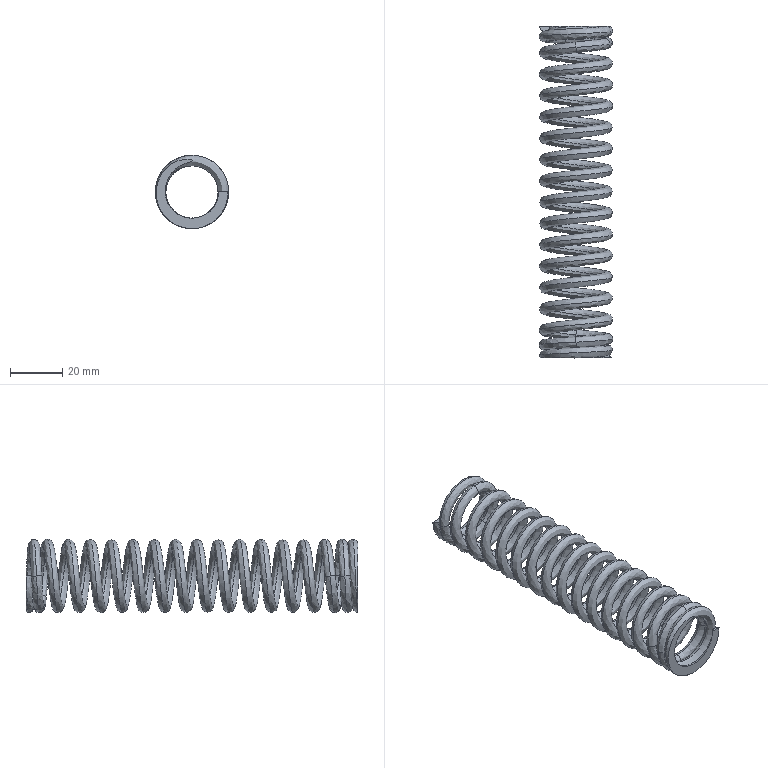Part | SolidWorks | features LayoutProfileFeature 1 | 1 solid | 26 faces | volume 16373 mm3 | spline 22 | plane 4